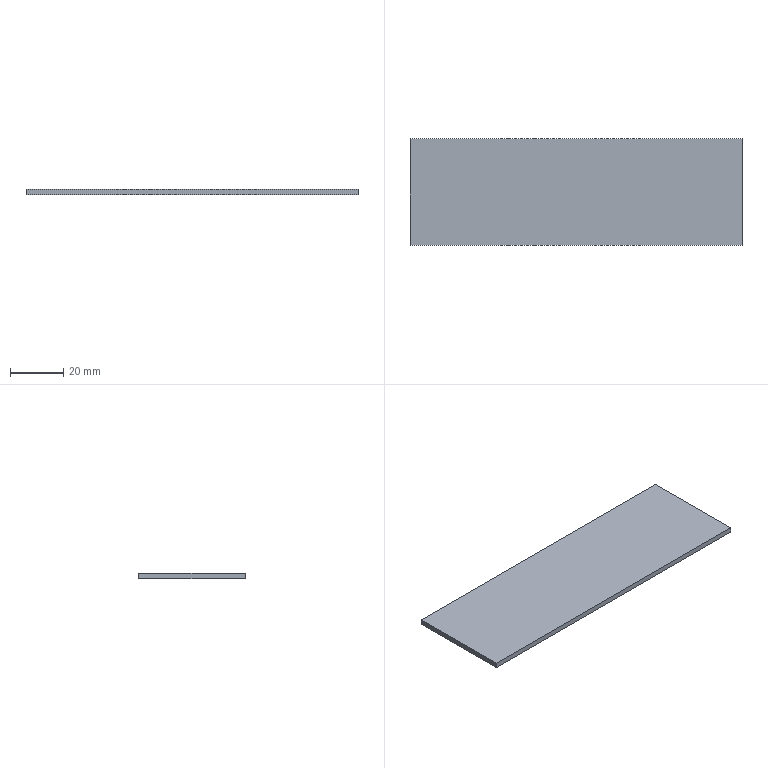Part | SolidWorks | features Extrusion 1 | 1 solid | 6 faces | box 125 x 40 x 2 mm | volume 10000 mm3 | plane 6
STEP:
#1=CARTESIAN_POINT('',(-62.5,20.,0.));
#2=VERTEX_POINT('',#1);
#3=CARTESIAN_POINT('',(-62.5,-20.,0.));
#4=VERTEX_POINT('',#3);
#5=CARTESIAN_POINT('',(-62.5,20.,0.));
#6=DIRECTION('',(0.,-1.,0.));
#7=VECTOR('',#6,1000.);
#8=LINE('',#5,#7);
#9=EDGE_CURVE('',#2,#4,#8,.T.);
#10=ORIENTED_EDGE('',*,*,#9,.T.);
#11=CARTESIAN_POINT('',(-62.5,-20.,2.));
#12=VERTEX_POINT('',#11);
#13=CARTESIAN_POINT('',(-62.5,-20.,2.));
#14=DIRECTION('',(0.,0.,-1.));
#15=VECTOR('',#14,1000.);
#16=LINE('',#13,#15);
#17=EDGE_CURVE('',#12,#4,#16,.T.);
#18=ORIENTED_EDGE('',*,*,#17,.F.);
#19=CARTESIAN_POINT('',(-62.5,20.,2.));
#20=VERTEX_POINT('',#19);
#21=CARTESIAN_POINT('',(-62.5,20.,2.));
#22=DIRECTION('',(0.,-1.,0.));
#23=VECTOR('',#22,1000.);
#24=LINE('',#21,#23);
#25=EDGE_CURVE('',#20,#12,#24,.T.);
#26=ORIENTED_EDGE('',*,*,#25,.F.);
#27=CARTESIAN_POINT('',(-62.5,20.,2.));
#28=DIRECTION('',(0.,0.,-1.));
#29=VECTOR('',#28,1000.);
#30=LINE('',#27,#29);
#31=EDGE_CURVE('',#20,#2,#30,.T.);
#32=ORIENTED_EDGE('',*,*,#31,.T.);
#33=EDGE_LOOP('',(#10,#18,#26,#32));
#34=FACE_OUTER_BOUND('',#33,.T.);
#35=CARTESIAN_POINT('',(-62.5,20.,2.));
#36=DIRECTION('',(1.,0.,0.));
#37=DIRECTION('',(0.,0.,-1.));
#38=AXIS2_PLACEMENT_3D('',#35,#36,#37);
#39=PLANE('',#38);
#40=ADVANCED_FACE('',(#34),#39,.F.);
#41=CARTESIAN_POINT('',(62.5,-20.,0.));
#42=VERTEX_POINT('',#41);
#43=CARTESIAN_POINT('',(-62.5,-20.,0.));
#44=DIRECTION('',(1.,0.,0.));
#45=VECTOR('',#44,1000.);
#46=LINE('',#43,#45);
#47=EDGE_CURVE('',#4,#42,#46,.T.);
#48=ORIENTED_EDGE('',*,*,#47,.T.);
#49=CARTESIAN_POINT('',(62.5,-20.,2.));
#50=VERTEX_POINT('',#49);
#51=CARTESIAN_POINT('',(62.5,-20.,2.));
#52=DIRECTION('',(0.,0.,-1.));
#53=VECTOR('',#52,1000.);
#54=LINE('',#51,#53);
#55=EDGE_CURVE('',#50,#42,#54,.T.);
#56=ORIENTED_EDGE('',*,*,#55,.F.);
#57=CARTESIAN_POINT('',(-62.5,-20.,2.));
#58=DIRECTION('',(1.,0.,0.));
#59=VECTOR('',#58,1000.);
#60=LINE('',#57,#59);
#61=EDGE_CURVE('',#12,#50,#60,.T.);
#62=ORIENTED_EDGE('',*,*,#61,.F.);
#63=ORIENTED_EDGE('',*,*,#17,.T.);
#64=EDGE_LOOP('',(#48,#56,#62,#63));
#65=FACE_OUTER_BOUND('',#64,.T.);
#66=CARTESIAN_POINT('',(-62.5,-20.,2.));
#67=DIRECTION('',(0.,1.,0.));
#68=DIRECTION('',(-1.,0.,0.));
#69=AXIS2_PLACEMENT_3D('',#66,#67,#68);
#70=PLANE('',#69);
#71=ADVANCED_FACE('',(#65),#70,.F.);
#72=CARTESIAN_POINT('',(62.5,20.,0.));
#73=VERTEX_POINT('',#72);
#74=CARTESIAN_POINT('',(62.5,20.,0.));
#75=DIRECTION('',(0.,1.,0.));
#76=VECTOR('',#75,1000.);
#77=LINE('',#74,#76);
#78=EDGE_CURVE('',#42,#73,#77,.T.);
#79=ORIENTED_EDGE('',*,*,#78,.T.);
#80=CARTESIAN_POINT('',(62.5,20.,2.));
#81=VERTEX_POINT('',#80);
#82=CARTESIAN_POINT('',(62.5,20.,2.));
#83=DIRECTION('',(0.,0.,-1.));
#84=VECTOR('',#83,1000.);
#85=LINE('',#82,#84);
#86=EDGE_CURVE('',#81,#73,#85,.T.);
#87=ORIENTED_EDGE('',*,*,#86,.F.);
#88=CARTESIAN_POINT('',(62.5,20.,2.));
#89=DIRECTION('',(0.,1.,0.));
#90=VECTOR('',#89,1000.);
#91=LINE('',#88,#90);
#92=EDGE_CURVE('',#50,#81,#91,.T.);
#93=ORIENTED_EDGE('',*,*,#92,.F.);
#94=ORIENTED_EDGE('',*,*,#55,.T.);
#95=EDGE_LOOP('',(#79,#87,#93,#94));
#96=FACE_OUTER_BOUND('',#95,.T.);
#97=CARTESIAN_POINT('',(62.5,20.,2.));
#98=DIRECTION('',(-1.,0.,0.));
#99=DIRECTION('',(0.,0.,1.));
#100=AXIS2_PLACEMENT_3D('',#97,#98,#99);
#101=PLANE('',#100);
#102=ADVANCED_FACE('',(#96),#101,.F.);
#103=CARTESIAN_POINT('',(-62.5,20.,0.));
#104=DIRECTION('',(-1.,0.,0.));
#105=VECTOR('',#104,1000.);
#106=LINE('',#103,#105);
#107=EDGE_CURVE('',#73,#2,#106,.T.);
#108=ORIENTED_EDGE('',*,*,#107,.T.);
#109=ORIENTED_EDGE('',*,*,#31,.F.);
#110=CARTESIAN_POINT('',(-62.5,20.,2.));
#111=DIRECTION('',(-1.,0.,0.));
#112=VECTOR('',#111,1000.);
#113=LINE('',#110,#112);
#114=EDGE_CURVE('',#81,#20,#113,.T.);
#115=ORIENTED_EDGE('',*,*,#114,.F.);
#116=ORIENTED_EDGE('',*,*,#86,.T.);
#117=EDGE_LOOP('',(#108,#109,#115,#116));
#118=FACE_OUTER_BOUND('',#117,.T.);
#119=CARTESIAN_POINT('',(-62.5,20.,2.));
#120=DIRECTION('',(0.,-1.,0.));
#121=DIRECTION('',(0.,0.,-1.));
#122=AXIS2_PLACEMENT_3D('',#119,#120,#121);
#123=PLANE('',#122);
#124=ADVANCED_FACE('',(#118),#123,.F.);
#125=ORIENTED_EDGE('',*,*,#25,.T.);
#126=ORIENTED_EDGE('',*,*,#61,.T.);
#127=ORIENTED_EDGE('',*,*,#92,.T.);
#128=ORIENTED_EDGE('',*,*,#114,.T.);
#129=EDGE_LOOP('',(#125,#126,#127,#128));
#130=FACE_OUTER_BOUND('',#129,.T.);
#131=CARTESIAN_POINT('',(0.,0.,2.));
#132=DIRECTION('',(0.,0.,1.));
#133=DIRECTION('',(1.,0.,0.));
#134=AXIS2_PLACEMENT_3D('',#131,#132,#133);
#135=PLANE('',#134);
#136=ADVANCED_FACE('',(#130),#135,.T.);
#137=ORIENTED_EDGE('',*,*,#9,.F.);
#138=ORIENTED_EDGE('',*,*,#107,.F.);
#139=ORIENTED_EDGE('',*,*,#78,.F.);
#140=ORIENTED_EDGE('',*,*,#47,.F.);
#141=EDGE_LOOP('',(#137,#138,#139,#140));
#142=FACE_OUTER_BOUND('',#141,.T.);
#143=CARTESIAN_POINT('',(0.,0.,0.));
#144=DIRECTION('',(0.,0.,1.));
#145=DIRECTION('',(1.,0.,0.));
#146=AXIS2_PLACEMENT_3D('',#143,#144,#145);
#147=PLANE('',#146);
#148=ADVANCED_FACE('',(#142),#147,.F.);
#149=CLOSED_SHELL('',(#40,#71,#102,#124,#136,#148));
#150=MANIFOLD_SOLID_BREP('',#149);
#151=CARTESIAN_POINT('',(0.,0.,0.));
#152=DIRECTION('',(0.,0.,1.));
#153=DIRECTION('',(1.,0.,0.));
#154=AXIS2_PLACEMENT_3D('',#151,#152,#153);
#155=(LENGTH_UNIT()NAMED_UNIT(*)SI_UNIT(.MILLI.,.METRE.));
#156=UNCERTAINTY_MEASURE_WITH_UNIT(LENGTH_MEASURE(0.00001),#155,'','');
#157=(NAMED_UNIT(*)PLANE_ANGLE_UNIT()SI_UNIT($,.RADIAN.));
#158=(NAMED_UNIT(*)SI_UNIT($,.STERADIAN.)SOLID_ANGLE_UNIT());
#159=(GEOMETRIC_REPRESENTATION_CONTEXT(3)GLOBAL_UNCERTAINTY_ASSIGNED_CONTEXT((#156))GLOBAL_UNIT_ASSIGNED_CONTEXT((#155,#157,#158))REPRESENTATION_CONTEXT('',''));
#160=ADVANCED_BREP_SHAPE_REPRESENTATION('',(#150,#154),#159);